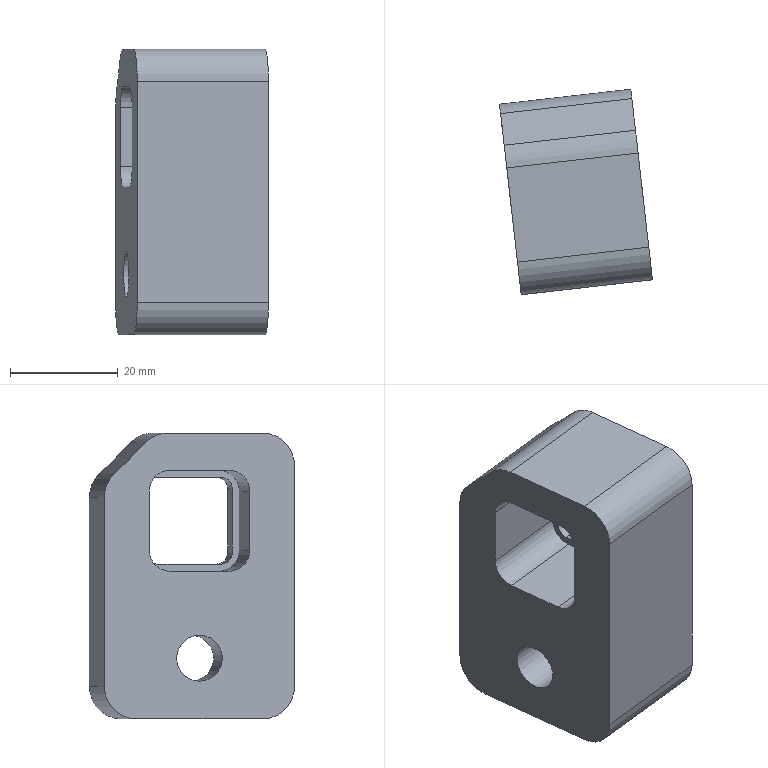Part | NX | features solid 2 | 1 solid | 32 faces | box 28.361 x 38.045 x 53 mm | volume 34321 mm3 | plane 17 | cylinder 15 | commonest cylinder face diameters 12 x5 4.08 x4 7.75 x4 8.5 x1 14 x1
STEP:
#1=CARTESIAN_POINT('',(3205.892,233.848,-55.317));
#2=VERTEX_POINT('',#1);
#3=CARTESIAN_POINT('',(3205.453,237.698,-51.442));
#4=VERTEX_POINT('',#3);
#5=CARTESIAN_POINT('',(3205.453,237.698,-55.317));
#6=DIRECTION('',(-0.9936,-0.1132,-0.000000001));
#7=DIRECTION('',(0.000000001,0.,-1.));
#8=AXIS2_PLACEMENT_3D('',#5,#6,#7);
#9=CIRCLE('',#8,3.875);
#10=EDGE_CURVE('',#2,#4,#9,.T.);
#11=ORIENTED_EDGE('',*,*,#10,.T.);
#12=CARTESIAN_POINT('',(3204.208,248.628,-51.442));
#13=VERTEX_POINT('',#12);
#14=CARTESIAN_POINT('',(3204.83,243.163,-51.442));
#15=DIRECTION('',(-0.1132,0.9936,0.));
#16=VECTOR('',#15,1000.);
#17=LINE('',#14,#16);
#18=EDGE_CURVE('',#4,#13,#17,.T.);
#19=ORIENTED_EDGE('',*,*,#18,.T.);
#20=CARTESIAN_POINT('',(3203.769,252.478,-55.317));
#21=VERTEX_POINT('',#20);
#22=CARTESIAN_POINT('',(3204.208,248.628,-55.317));
#23=DIRECTION('',(-0.9936,-0.1132,-0.000000001));
#24=DIRECTION('',(0.000000001,0.,-1.));
#25=AXIS2_PLACEMENT_3D('',#22,#23,#24);
#26=CIRCLE('',#25,3.875);
#27=EDGE_CURVE('',#13,#21,#26,.T.);
#28=ORIENTED_EDGE('',*,*,#27,.T.);
#29=CARTESIAN_POINT('',(3203.769,252.478,-66.317));
#30=VERTEX_POINT('',#29);
#31=CARTESIAN_POINT('',(3203.769,252.478,-61.567));
#32=DIRECTION('',(0.000000001,0.,-1.));
#33=VECTOR('',#32,1000.);
#34=LINE('',#31,#33);
#35=EDGE_CURVE('',#21,#30,#34,.T.);
#36=ORIENTED_EDGE('',*,*,#35,.T.);
#37=CARTESIAN_POINT('',(3204.208,248.628,-70.192));
#38=VERTEX_POINT('',#37);
#39=CARTESIAN_POINT('',(3204.208,248.628,-66.317));
#40=DIRECTION('',(0.9936,0.1132,0.000000001));
#41=DIRECTION('',(0.000000001,0.,-1.));
#42=AXIS2_PLACEMENT_3D('',#39,#40,#41);
#43=CIRCLE('',#42,3.875);
#44=EDGE_CURVE('',#38,#30,#43,.T.);
#45=ORIENTED_EDGE('',*,*,#44,.F.);
#46=CARTESIAN_POINT('',(3205.453,237.698,-70.192));
#47=VERTEX_POINT('',#46);
#48=CARTESIAN_POINT('',(3204.208,248.628,-70.192));
#49=DIRECTION('',(-0.1132,0.9936,0.));
#50=VECTOR('',#49,1000.);
#51=LINE('',#48,#50);
#52=EDGE_CURVE('',#47,#38,#51,.T.);
#53=ORIENTED_EDGE('',*,*,#52,.F.);
#54=CARTESIAN_POINT('',(3205.892,233.848,-66.317));
#55=VERTEX_POINT('',#54);
#56=CARTESIAN_POINT('',(3205.453,237.698,-66.317));
#57=DIRECTION('',(0.9936,0.1132,0.000000001));
#58=DIRECTION('',(0.000000001,0.,-1.));
#59=AXIS2_PLACEMENT_3D('',#56,#57,#58);
#60=CIRCLE('',#59,3.875);
#61=EDGE_CURVE('',#55,#47,#60,.T.);
#62=ORIENTED_EDGE('',*,*,#61,.F.);
#63=CARTESIAN_POINT('',(3205.892,233.848,-66.317));
#64=DIRECTION('',(0.000000001,0.,-1.));
#65=VECTOR('',#64,1000.);
#66=LINE('',#63,#65);
#67=EDGE_CURVE('',#2,#55,#66,.T.);
#68=ORIENTED_EDGE('',*,*,#67,.F.);
#69=EDGE_LOOP('',(#11,#19,#28,#36,#45,#53,#62,#68));
#70=FACE_BOUND('',#69,.T.);
#71=CARTESIAN_POINT('',(3205.74,235.175,-66.817));
#72=VERTEX_POINT('',#71);
#73=CARTESIAN_POINT('',(3205.74,235.175,-54.817));
#74=VERTEX_POINT('',#73);
#75=CARTESIAN_POINT('',(3205.74,235.175,-54.817));
#76=DIRECTION('',(-0.000000001,0.000000001,1.));
#77=VECTOR('',#76,1000.);
#78=LINE('',#75,#77);
#79=EDGE_CURVE('',#72,#74,#78,.T.);
#80=ORIENTED_EDGE('',*,*,#79,.F.);
#81=CARTESIAN_POINT('',(3205.51,237.202,-68.857));
#82=VERTEX_POINT('',#81);
#83=CARTESIAN_POINT('',(3205.51,237.202,-66.817));
#84=DIRECTION('',(-0.9936,-0.1132,-0.000000001));
#85=DIRECTION('',(0.000000001,0.,-1.));
#86=AXIS2_PLACEMENT_3D('',#83,#84,#85);
#87=CIRCLE('',#86,2.04);
#88=EDGE_CURVE('',#82,#72,#87,.T.);
#89=ORIENTED_EDGE('',*,*,#88,.F.);
#90=CARTESIAN_POINT('',(3204.151,249.124,-68.857));
#91=VERTEX_POINT('',#90);
#92=CARTESIAN_POINT('',(3205.51,237.202,-68.857));
#93=DIRECTION('',(0.1132,-0.9936,0.000000001));
#94=VECTOR('',#93,1000.);
#95=LINE('',#92,#94);
#96=EDGE_CURVE('',#91,#82,#95,.T.);
#97=ORIENTED_EDGE('',*,*,#96,.F.);
#98=CARTESIAN_POINT('',(3203.92,251.151,-66.817));
#99=VERTEX_POINT('',#98);
#100=CARTESIAN_POINT('',(3204.151,249.124,-66.817));
#101=DIRECTION('',(-0.9936,-0.1132,-0.000000001));
#102=DIRECTION('',(0.000000001,0.,-1.));
#103=AXIS2_PLACEMENT_3D('',#100,#101,#102);
#104=CIRCLE('',#103,2.04);
#105=EDGE_CURVE('',#99,#91,#104,.T.);
#106=ORIENTED_EDGE('',*,*,#105,.F.);
#107=CARTESIAN_POINT('',(3203.92,251.151,-54.817));
#108=VERTEX_POINT('',#107);
#109=CARTESIAN_POINT('',(3203.92,251.151,-66.317));
#110=DIRECTION('',(0.000000001,0.,-1.));
#111=VECTOR('',#110,1000.);
#112=LINE('',#109,#111);
#113=EDGE_CURVE('',#108,#99,#112,.T.);
#114=ORIENTED_EDGE('',*,*,#113,.F.);
#115=CARTESIAN_POINT('',(3204.151,249.124,-52.777));
#116=VERTEX_POINT('',#115);
#117=CARTESIAN_POINT('',(3204.151,249.124,-54.817));
#118=DIRECTION('',(-0.9936,-0.1132,-0.000000001));
#119=DIRECTION('',(0.000000001,0.,-1.));
#120=AXIS2_PLACEMENT_3D('',#117,#118,#119);
#121=CIRCLE('',#120,2.04);
#122=EDGE_CURVE('',#116,#108,#121,.T.);
#123=ORIENTED_EDGE('',*,*,#122,.F.);
#124=CARTESIAN_POINT('',(3205.51,237.202,-52.777));
#125=VERTEX_POINT('',#124);
#126=CARTESIAN_POINT('',(3204.151,249.124,-52.777));
#127=DIRECTION('',(-0.1132,0.9936,-0.000000001));
#128=VECTOR('',#127,1000.);
#129=LINE('',#126,#128);
#130=EDGE_CURVE('',#125,#116,#129,.T.);
#131=ORIENTED_EDGE('',*,*,#130,.F.);
#132=CARTESIAN_POINT('',(3205.51,237.202,-54.817));
#133=DIRECTION('',(-0.9936,-0.1132,-0.000000001));
#134=DIRECTION('',(0.000000001,0.,-1.));
#135=AXIS2_PLACEMENT_3D('',#132,#133,#134);
#136=CIRCLE('',#135,2.04);
#137=EDGE_CURVE('',#74,#125,#136,.T.);
#138=ORIENTED_EDGE('',*,*,#137,.F.);
#139=EDGE_LOOP('',(#80,#89,#97,#106,#114,#123,#131,#138));
#140=FACE_BOUND('',#139,.T.);
#141=CARTESIAN_POINT('',(3204.83,243.163,-61.567));
#142=DIRECTION('',(-0.9936,-0.1132,-0.000000001));
#143=DIRECTION('',(-0.1132,0.9936,0.));
#144=AXIS2_PLACEMENT_3D('',#141,#142,#143);
#145=PLANE('',#144);
#146=ADVANCED_FACE('',(#70,#140),#145,.T.);
#147=CARTESIAN_POINT('',(3187.94,241.239,-90.567));
#148=VERTEX_POINT('',#147);
#149=CARTESIAN_POINT('',(3187.94,241.239,-86.317));
#150=DIRECTION('',(-0.9936,-0.1132,-0.000000001));
#151=DIRECTION('',(0.000000001,0.,-1.));
#152=AXIS2_PLACEMENT_3D('',#149,#150,#151);
#153=CIRCLE('',#152,4.25);
#154=EDGE_CURVE('',#148,#148,#153,.T.);
#155=ORIENTED_EDGE('',*,*,#154,.F.);
#156=EDGE_LOOP('',(#155));
#157=FACE_BOUND('',#156,.T.);
#158=CARTESIAN_POINT('',(3189.27,229.564,-44.567));
#159=VERTEX_POINT('',#158);
#160=CARTESIAN_POINT('',(3187.279,247.036,-44.567));
#161=VERTEX_POINT('',#160);
#162=CARTESIAN_POINT('',(3189.921,223.851,-44.567));
#163=DIRECTION('',(-0.1132,0.9936,0.));
#164=VECTOR('',#163,1000.);
#165=LINE('',#162,#164);
#166=EDGE_CURVE('',#159,#161,#165,.T.);
#167=ORIENTED_EDGE('',*,*,#166,.T.);
#168=CARTESIAN_POINT('',(3186.799,251.252,-46.324));
#169=VERTEX_POINT('',#168);
#170=CARTESIAN_POINT('',(3187.279,247.036,-50.567));
#171=DIRECTION('',(0.9936,0.1132,0.000000001));
#172=DIRECTION('',(0.000000001,0.,-1.));
#173=AXIS2_PLACEMENT_3D('',#170,#171,#172);
#174=CIRCLE('',#173,6.);
#175=EDGE_CURVE('',#169,#161,#174,.T.);
#176=ORIENTED_EDGE('',*,*,#175,.F.);
#177=CARTESIAN_POINT('',(3186.129,257.128,-52.239));
#178=VERTEX_POINT('',#177);
#179=CARTESIAN_POINT('',(3186.506,253.817,-48.907));
#180=DIRECTION('',(0.08005,-0.7026,0.7071));
#181=VECTOR('',#180,1000.);
#182=LINE('',#179,#181);
#183=EDGE_CURVE('',#178,#169,#182,.T.);
#184=ORIENTED_EDGE('',*,*,#183,.F.);
#185=CARTESIAN_POINT('',(3185.93,258.874,-56.482));
#186=VERTEX_POINT('',#185);
#187=CARTESIAN_POINT('',(3186.609,252.913,-56.482));
#188=DIRECTION('',(0.9936,0.1132,0.000000001));
#189=DIRECTION('',(0.000000001,0.,-1.));
#190=AXIS2_PLACEMENT_3D('',#187,#188,#189);
#191=CIRCLE('',#190,6.);
#192=EDGE_CURVE('',#186,#178,#191,.T.);
#193=ORIENTED_EDGE('',*,*,#192,.F.);
#194=CARTESIAN_POINT('',(3185.93,258.874,-91.567));
#195=VERTEX_POINT('',#194);
#196=CARTESIAN_POINT('',(3185.93,258.874,-61.567));
#197=DIRECTION('',(-0.000000001,0.,1.));
#198=VECTOR('',#197,1000.);
#199=LINE('',#196,#198);
#200=EDGE_CURVE('',#195,#186,#199,.T.);
#201=ORIENTED_EDGE('',*,*,#200,.F.);
#202=CARTESIAN_POINT('',(3186.609,252.913,-97.567));
#203=VERTEX_POINT('',#202);
#204=CARTESIAN_POINT('',(3186.609,252.913,-91.567));
#205=DIRECTION('',(0.9936,0.1132,0.000000001));
#206=DIRECTION('',(0.000000001,0.,-1.));
#207=AXIS2_PLACEMENT_3D('',#204,#205,#206);
#208=CIRCLE('',#207,6.);
#209=EDGE_CURVE('',#203,#195,#208,.T.);
#210=ORIENTED_EDGE('',*,*,#209,.F.);
#211=CARTESIAN_POINT('',(3189.27,229.564,-97.567));
#212=VERTEX_POINT('',#211);
#213=CARTESIAN_POINT('',(3187.94,241.239,-97.567));
#214=DIRECTION('',(-0.1132,0.9936,0.));
#215=VECTOR('',#214,1000.);
#216=LINE('',#213,#215);
#217=EDGE_CURVE('',#212,#203,#216,.T.);
#218=ORIENTED_EDGE('',*,*,#217,.F.);
#219=CARTESIAN_POINT('',(3189.949,223.603,-91.567));
#220=VERTEX_POINT('',#219);
#221=CARTESIAN_POINT('',(3189.27,229.564,-91.567));
#222=DIRECTION('',(0.9936,0.1132,0.000000001));
#223=DIRECTION('',(0.000000001,0.,-1.));
#224=AXIS2_PLACEMENT_3D('',#221,#222,#223);
#225=CIRCLE('',#224,6.);
#226=EDGE_CURVE('',#220,#212,#225,.T.);
#227=ORIENTED_EDGE('',*,*,#226,.F.);
#228=CARTESIAN_POINT('',(3189.949,223.603,-50.567));
#229=VERTEX_POINT('',#228);
#230=CARTESIAN_POINT('',(3189.949,223.603,-61.567));
#231=DIRECTION('',(0.000000001,0.,-1.));
#232=VECTOR('',#231,1000.);
#233=LINE('',#230,#232);
#234=EDGE_CURVE('',#229,#220,#233,.T.);
#235=ORIENTED_EDGE('',*,*,#234,.F.);
#236=CARTESIAN_POINT('',(3189.27,229.564,-50.567));
#237=DIRECTION('',(0.9936,0.1132,0.000000001));
#238=DIRECTION('',(0.000000001,0.,-1.));
#239=AXIS2_PLACEMENT_3D('',#236,#237,#238);
#240=CIRCLE('',#239,6.);
#241=EDGE_CURVE('',#159,#229,#240,.T.);
#242=ORIENTED_EDGE('',*,*,#241,.F.);
#243=EDGE_LOOP('',(#167,#176,#184,#193,#201,#210,#218,#227,#235,#242));
#244=FACE_BOUND('',#243,.T.);
#245=CARTESIAN_POINT('',(3187.317,246.703,-70.192));
#246=VERTEX_POINT('',#245);
#247=CARTESIAN_POINT('',(3186.878,250.553,-66.317));
#248=VERTEX_POINT('',#247);
#249=CARTESIAN_POINT('',(3187.317,246.703,-66.317));
#250=DIRECTION('',(0.9936,0.1132,0.000000001));
#251=DIRECTION('',(0.000000001,0.,-1.));
#252=AXIS2_PLACEMENT_3D('',#249,#250,#251);
#253=CIRCLE('',#252,3.875);
#254=EDGE_CURVE('',#246,#248,#253,.T.);
#255=ORIENTED_EDGE('',*,*,#254,.T.);
#256=CARTESIAN_POINT('',(3186.878,250.553,-55.317));
#257=VERTEX_POINT('',#256);
#258=CARTESIAN_POINT('',(3186.878,250.553,-61.567));
#259=DIRECTION('',(0.000000001,0.,-1.));
#260=VECTOR('',#259,1000.);
#261=LINE('',#258,#260);
#262=EDGE_CURVE('',#257,#248,#261,.T.);
#263=ORIENTED_EDGE('',*,*,#262,.F.);
#264=CARTESIAN_POINT('',(3187.317,246.703,-51.442));
#265=VERTEX_POINT('',#264);
#266=CARTESIAN_POINT('',(3187.317,246.703,-55.317));
#267=DIRECTION('',(0.9936,0.1132,0.000000001));
#268=DIRECTION('',(0.000000001,0.,-1.));
#269=AXIS2_PLACEMENT_3D('',#266,#267,#268);
#270=CIRCLE('',#269,3.875);
#271=EDGE_CURVE('',#257,#265,#270,.T.);
#272=ORIENTED_EDGE('',*,*,#271,.T.);
#273=CARTESIAN_POINT('',(3188.562,235.774,-51.442));
#274=VERTEX_POINT('',#273);
#275=CARTESIAN_POINT('',(3187.94,241.239,-51.442));
#276=DIRECTION('',(-0.1132,0.9936,0.));
#277=VECTOR('',#276,1000.);
#278=LINE('',#275,#277);
#279=EDGE_CURVE('',#274,#265,#278,.T.);
#280=ORIENTED_EDGE('',*,*,#279,.F.);
#281=CARTESIAN_POINT('',(3189.001,231.924,-55.317));
#282=VERTEX_POINT('',#281);
#283=CARTESIAN_POINT('',(3188.562,235.774,-55.317));
#284=DIRECTION('',(0.9936,0.1132,0.000000001));
#285=DIRECTION('',(0.000000001,0.,-1.));
#286=AXIS2_PLACEMENT_3D('',#283,#284,#285);
#287=CIRCLE('',#286,3.875);
#288=EDGE_CURVE('',#274,#282,#287,.T.);
#289=ORIENTED_EDGE('',*,*,#288,.T.);
#290=CARTESIAN_POINT('',(3189.001,231.924,-66.317));
#291=VERTEX_POINT('',#290);
#292=CARTESIAN_POINT('',(3189.001,231.924,-61.567));
#293=DIRECTION('',(-0.000000001,0.,1.));
#294=VECTOR('',#293,1000.);
#295=LINE('',#292,#294);
#296=EDGE_CURVE('',#291,#282,#295,.T.);
#297=ORIENTED_EDGE('',*,*,#296,.F.);
#298=CARTESIAN_POINT('',(3188.562,235.774,-70.192));
#299=VERTEX_POINT('',#298);
#300=CARTESIAN_POINT('',(3188.562,235.774,-66.317));
#301=DIRECTION('',(0.9936,0.1132,0.000000001));
#302=DIRECTION('',(0.000000001,0.,-1.));
#303=AXIS2_PLACEMENT_3D('',#300,#301,#302);
#304=CIRCLE('',#303,3.875);
#305=EDGE_CURVE('',#291,#299,#304,.T.);
#306=ORIENTED_EDGE('',*,*,#305,.T.);
#307=CARTESIAN_POINT('',(3187.94,241.239,-70.192));
#308=DIRECTION('',(0.1132,-0.9936,0.));
#309=VECTOR('',#308,1000.);
#310=LINE('',#307,#309);
#311=EDGE_CURVE('',#246,#299,#310,.T.);
#312=ORIENTED_EDGE('',*,*,#311,.F.);
#313=EDGE_LOOP('',(#255,#263,#272,#280,#289,#297,#306,#312));
#314=FACE_BOUND('',#313,.T.);
#315=CARTESIAN_POINT('',(3187.94,241.239,-61.567));
#316=DIRECTION('',(-0.9936,-0.1132,-0.000000001));
#317=DIRECTION('',(-0.1132,0.9936,0.));
#318=AXIS2_PLACEMENT_3D('',#315,#316,#317);
#319=PLANE('',#318);
#320=ADVANCED_FACE('',(#157,#244,#314),#319,.T.);
#321=CARTESIAN_POINT('',(3212.961,238.051,-52.777));
#322=VERTEX_POINT('',#321);
#323=CARTESIAN_POINT('',(3211.603,249.973,-52.777));
#324=VERTEX_POINT('',#323);
#325=CARTESIAN_POINT('',(3214.263,226.624,-52.777));
#326=DIRECTION('',(-0.1132,0.9936,-0.000000001));
#327=VECTOR('',#326,1000.);
#328=LINE('',#325,#327);
#329=EDGE_CURVE('',#322,#324,#328,.T.);
#330=ORIENTED_EDGE('',*,*,#329,.T.);
#331=CARTESIAN_POINT('',(3211.372,252.,-54.817));
#332=VERTEX_POINT('',#331);
#333=CARTESIAN_POINT('',(3211.603,249.973,-54.817));
#334=DIRECTION('',(-0.9936,-0.1132,-0.000000001));
#335=DIRECTION('',(-0.000000001,0.,1.));
#336=AXIS2_PLACEMENT_3D('',#333,#334,#335);
#337=CIRCLE('',#336,2.04);
#338=EDGE_CURVE('',#324,#332,#337,.T.);
#339=ORIENTED_EDGE('',*,*,#338,.T.);
#340=CARTESIAN_POINT('',(3211.372,252.,-66.817));
#341=VERTEX_POINT('',#340);
#342=CARTESIAN_POINT('',(3211.372,252.,-70.067));
#343=DIRECTION('',(0.000000001,0.,-1.));
#344=VECTOR('',#343,1000.);
#345=LINE('',#342,#344);
#346=EDGE_CURVE('',#332,#341,#345,.T.);
#347=ORIENTED_EDGE('',*,*,#346,.T.);
#348=CARTESIAN_POINT('',(3211.603,249.973,-68.857));
#349=VERTEX_POINT('',#348);
#350=CARTESIAN_POINT('',(3211.603,249.973,-66.817));
#351=DIRECTION('',(-0.9936,-0.1132,-0.000000001));
#352=DIRECTION('',(-0.000000001,0.,1.));
#353=AXIS2_PLACEMENT_3D('',#350,#351,#352);
#354=CIRCLE('',#353,2.04);
#355=EDGE_CURVE('',#341,#349,#354,.T.);
#356=ORIENTED_EDGE('',*,*,#355,.T.);
#357=CARTESIAN_POINT('',(3212.961,238.051,-68.857));
#358=VERTEX_POINT('',#357);
#359=CARTESIAN_POINT('',(3214.263,226.624,-68.857));
#360=DIRECTION('',(0.1132,-0.9936,0.000000001));
#361=VECTOR('',#360,1000.);
#362=LINE('',#359,#361);
#363=EDGE_CURVE('',#349,#358,#362,.T.);
#364=ORIENTED_EDGE('',*,*,#363,.T.);
#365=CARTESIAN_POINT('',(3213.192,236.024,-66.817));
#366=VERTEX_POINT('',#365);
#367=CARTESIAN_POINT('',(3212.961,238.051,-66.817));
#368=DIRECTION('',(-0.9936,-0.1132,-0.000000001));
#369=DIRECTION('',(-0.000000001,0.,1.));
#370=AXIS2_PLACEMENT_3D('',#367,#368,#369);
#371=CIRCLE('',#370,2.04);
#372=EDGE_CURVE('',#358,#366,#371,.T.);
#373=ORIENTED_EDGE('',*,*,#372,.T.);
#374=CARTESIAN_POINT('',(3213.192,236.024,-54.817));
#375=VERTEX_POINT('',#374);
#376=CARTESIAN_POINT('',(3213.192,236.024,-70.067));
#377=DIRECTION('',(-0.000000001,0.000000001,1.));
#378=VECTOR('',#377,1000.);
#379=LINE('',#376,#378);
#380=EDGE_CURVE('',#366,#375,#379,.T.);
#381=ORIENTED_EDGE('',*,*,#380,.T.);
#382=CARTESIAN_POINT('',(3212.961,238.051,-54.817));
#383=DIRECTION('',(-0.9936,-0.1132,-0.000000001));
#384=DIRECTION('',(-0.000000001,0.,1.));
#385=AXIS2_PLACEMENT_3D('',#382,#383,#384);
#386=CIRCLE('',#385,2.04);
#387=EDGE_CURVE('',#375,#322,#386,.T.);
#388=ORIENTED_EDGE('',*,*,#387,.T.);
#389=EDGE_LOOP('',(#330,#339,#347,#356,#364,#373,#381,#388));
#390=FACE_BOUND('',#389,.T.);
#391=CARTESIAN_POINT('',(3214.291,226.376,-91.567));
#392=VERTEX_POINT('',#391);
#393=CARTESIAN_POINT('',(3214.291,226.376,-50.567));
#394=VERTEX_POINT('',#393);
#395=CARTESIAN_POINT('',(3214.291,226.376,-70.067));
#396=DIRECTION('',(-0.000000001,0.,1.));
#397=VECTOR('',#396,1000.);
#398=LINE('',#395,#397);
#399=EDGE_CURVE('',#392,#394,#398,.T.);
#400=ORIENTED_EDGE('',*,*,#399,.F.);
#401=CARTESIAN_POINT('',(3213.612,232.338,-97.567));
#402=VERTEX_POINT('',#401);
#403=CARTESIAN_POINT('',(3213.612,232.338,-91.567));
#404=DIRECTION('',(-0.9936,-0.1132,-0.000000001));
#405=DIRECTION('',(-0.000000001,0.,1.));
#406=AXIS2_PLACEMENT_3D('',#403,#404,#405);
#407=CIRCLE('',#406,6.);
#408=EDGE_CURVE('',#402,#392,#407,.T.);
#409=ORIENTED_EDGE('',*,*,#408,.F.);
#410=CARTESIAN_POINT('',(3210.952,255.686,-97.567));
#411=VERTEX_POINT('',#410);
#412=CARTESIAN_POINT('',(3214.263,226.624,-97.567));
#413=DIRECTION('',(-0.1132,0.9936,0.));
#414=VECTOR('',#413,1000.);
#415=LINE('',#412,#414);
#416=EDGE_CURVE('',#402,#411,#415,.T.);
#417=ORIENTED_EDGE('',*,*,#416,.T.);
#418=CARTESIAN_POINT('',(3210.273,261.648,-91.567));
#419=VERTEX_POINT('',#418);
#420=CARTESIAN_POINT('',(3210.952,255.686,-91.567));
#421=DIRECTION('',(-0.9936,-0.1132,-0.000000001));
#422=DIRECTION('',(-0.000000001,0.,1.));
#423=AXIS2_PLACEMENT_3D('',#420,#421,#422);
#424=CIRCLE('',#423,6.);
#425=EDGE_CURVE('',#419,#411,#424,.T.);
#426=ORIENTED_EDGE('',*,*,#425,.F.);
#427=CARTESIAN_POINT('',(3210.273,261.648,-56.482));
#428=VERTEX_POINT('',#427);
#429=CARTESIAN_POINT('',(3210.273,261.648,-70.067));
#430=DIRECTION('',(0.000000001,0.,-1.));
#431=VECTOR('',#430,1000.);
#432=LINE('',#429,#431);
#433=EDGE_CURVE('',#428,#419,#432,.T.);
#434=ORIENTED_EDGE('',*,*,#433,.F.);
#435=CARTESIAN_POINT('',(3210.472,259.902,-52.239));
#436=VERTEX_POINT('',#435);
#437=CARTESIAN_POINT('',(3210.952,255.686,-56.482));
#438=DIRECTION('',(-0.9936,-0.1132,-0.000000001));
#439=DIRECTION('',(-0.000000001,0.,1.));
#440=AXIS2_PLACEMENT_3D('',#437,#438,#439);
#441=CIRCLE('',#440,6.);
#442=EDGE_CURVE('',#436,#428,#441,.T.);
#443=ORIENTED_EDGE('',*,*,#442,.F.);
#444=CARTESIAN_POINT('',(3211.141,254.025,-46.324));
#445=VERTEX_POINT('',#444);
#446=CARTESIAN_POINT('',(3211.358,252.12,-44.407));
#447=DIRECTION('',(-0.08005,0.7026,-0.7071));
#448=VECTOR('',#447,1000.);
#449=LINE('',#446,#448);
#450=EDGE_CURVE('',#445,#436,#449,.T.);
#451=ORIENTED_EDGE('',*,*,#450,.F.);
#452=CARTESIAN_POINT('',(3211.622,249.81,-44.567));
#453=VERTEX_POINT('',#452);
#454=CARTESIAN_POINT('',(3211.622,249.81,-50.567));
#455=DIRECTION('',(-0.9936,-0.1132,-0.000000001));
#456=DIRECTION('',(-0.000000001,0.,1.));
#457=AXIS2_PLACEMENT_3D('',#454,#455,#456);
#458=CIRCLE('',#457,6.);
#459=EDGE_CURVE('',#453,#445,#458,.T.);
#460=ORIENTED_EDGE('',*,*,#459,.F.);
#461=CARTESIAN_POINT('',(3213.612,232.338,-44.567));
#462=VERTEX_POINT('',#461);
#463=CARTESIAN_POINT('',(3214.263,226.624,-44.567));
#464=DIRECTION('',(-0.1132,0.9936,0.));
#465=VECTOR('',#464,1000.);
#466=LINE('',#463,#465);
#467=EDGE_CURVE('',#462,#453,#466,.T.);
#468=ORIENTED_EDGE('',*,*,#467,.F.);
#469=CARTESIAN_POINT('',(3213.612,232.338,-50.567));
#470=DIRECTION('',(-0.9936,-0.1132,-0.000000001));
#471=DIRECTION('',(-0.000000001,0.,1.));
#472=AXIS2_PLACEMENT_3D('',#469,#470,#471);
#473=CIRCLE('',#472,6.);
#474=EDGE_CURVE('',#394,#462,#473,.T.);
#475=ORIENTED_EDGE('',*,*,#474,.F.);
#476=EDGE_LOOP('',(#400,#409,#417,#426,#434,#443,#451,#460,#468,#475));
#477=FACE_BOUND('',#476,.T.);
#478=CARTESIAN_POINT('',(3212.282,244.012,-79.317));
#479=VERTEX_POINT('',#478);
#480=CARTESIAN_POINT('',(3212.282,244.012,-86.317));
#481=DIRECTION('',(-0.9936,-0.1132,-0.000000001));
#482=DIRECTION('',(-0.000000001,0.,1.));
#483=AXIS2_PLACEMENT_3D('',#480,#481,#482);
#484=CIRCLE('',#483,7.);
#485=EDGE_CURVE('',#479,#479,#484,.T.);
#486=ORIENTED_EDGE('',*,*,#485,.T.);
#487=EDGE_LOOP('',(#486));
#488=FACE_BOUND('',#487,.T.);
#489=CARTESIAN_POINT('',(3214.263,226.624,-70.067));
#490=DIRECTION('',(0.9936,0.1132,0.000000001));
#491=DIRECTION('',(0.1132,-0.9936,0.));
#492=AXIS2_PLACEMENT_3D('',#489,#490,#491);
#493=PLANE('',#492);
#494=ADVANCED_FACE('',(#390,#477,#488),#493,.T.);
#495=ORIENTED_EDGE('',*,*,#200,.T.);
#496=CARTESIAN_POINT('',(3203.318,260.855,-56.482));
#497=DIRECTION('',(-0.9936,-0.1132,-0.000000001));
#498=VECTOR('',#497,1000.);
#499=LINE('',#496,#498);
#500=EDGE_CURVE('',#428,#186,#499,.T.);
#501=ORIENTED_EDGE('',*,*,#500,.F.);
#502=ORIENTED_EDGE('',*,*,#433,.T.);
#503=CARTESIAN_POINT('',(3203.318,260.855,-91.567));
#504=DIRECTION('',(0.9936,0.1132,0.000000001));
#505=VECTOR('',#504,1000.);
#506=LINE('',#503,#505);
#507=EDGE_CURVE('',#195,#419,#506,.T.);
#508=ORIENTED_EDGE('',*,*,#507,.F.);
#509=EDGE_LOOP('',(#495,#501,#502,#508));
#510=FACE_BOUND('',#509,.T.);
#511=CARTESIAN_POINT('',(3203.318,260.855,-70.067));
#512=DIRECTION('',(-0.1132,0.9936,0.));
#513=DIRECTION('',(0.9936,0.1132,0.000000001));
#514=AXIS2_PLACEMENT_3D('',#511,#512,#513);
#515=PLANE('',#514);
#516=ADVANCED_FACE('',(#510),#515,.T.);
#517=ORIENTED_EDGE('',*,*,#217,.T.);
#518=CARTESIAN_POINT('',(3203.997,254.894,-97.567));
#519=DIRECTION('',(-0.9936,-0.1132,-0.000000001));
#520=VECTOR('',#519,1000.);
#521=LINE('',#518,#520);
#522=EDGE_CURVE('',#411,#203,#521,.T.);
#523=ORIENTED_EDGE('',*,*,#522,.F.);
#524=ORIENTED_EDGE('',*,*,#416,.F.);
#525=CARTESIAN_POINT('',(3206.657,231.545,-97.567));
#526=DIRECTION('',(0.9936,0.1132,0.000000001));
#527=VECTOR('',#526,1000.);
#528=LINE('',#525,#527);
#529=EDGE_CURVE('',#212,#402,#528,.T.);
#530=ORIENTED_EDGE('',*,*,#529,.F.);
#531=EDGE_LOOP('',(#517,#523,#524,#530));
#532=FACE_BOUND('',#531,.T.);
#533=CARTESIAN_POINT('',(3207.308,225.832,-97.567));
#534=DIRECTION('',(0.000000001,0.,-1.));
#535=DIRECTION('',(0.1132,-0.9936,0.));
#536=AXIS2_PLACEMENT_3D('',#533,#534,#535);
#537=PLANE('',#536);
#538=ADVANCED_FACE('',(#532),#537,.T.);
#539=ORIENTED_EDGE('',*,*,#467,.T.);
#540=CARTESIAN_POINT('',(3204.667,249.017,-44.567));
#541=DIRECTION('',(0.9936,0.1132,0.000000001));
#542=VECTOR('',#541,1000.);
#543=LINE('',#540,#542);
#544=EDGE_CURVE('',#161,#453,#543,.T.);
#545=ORIENTED_EDGE('',*,*,#544,.F.);
#546=ORIENTED_EDGE('',*,*,#166,.F.);
#547=CARTESIAN_POINT('',(3206.657,231.545,-44.567));
#548=DIRECTION('',(-0.9936,-0.1132,-0.000000001));
#549=VECTOR('',#548,1000.);
#550=LINE('',#547,#549);
#551=EDGE_CURVE('',#462,#159,#550,.T.);
#552=ORIENTED_EDGE('',*,*,#551,.F.);
#553=EDGE_LOOP('',(#539,#545,#546,#552));
#554=FACE_BOUND('',#553,.T.);
#555=CARTESIAN_POINT('',(3207.308,225.832,-44.567));
#556=DIRECTION('',(-0.000000001,0.,1.));
#557=DIRECTION('',(-0.1132,0.9936,0.));
#558=AXIS2_PLACEMENT_3D('',#555,#556,#557);
#559=PLANE('',#558);
#560=ADVANCED_FACE('',(#554),#559,.T.);
#561=ORIENTED_EDGE('',*,*,#234,.T.);
#562=CARTESIAN_POINT('',(3207.336,225.584,-91.567));
#563=DIRECTION('',(-0.9936,-0.1132,-0.000000001));
#564=VECTOR('',#563,1000.);
#565=LINE('',#562,#564);
#566=EDGE_CURVE('',#392,#220,#565,.T.);
#567=ORIENTED_EDGE('',*,*,#566,.F.);
#568=ORIENTED_EDGE('',*,*,#399,.T.);
#569=CARTESIAN_POINT('',(3207.336,225.584,-50.567));
#570=DIRECTION('',(0.9936,0.1132,0.000000001));
#571=VECTOR('',#570,1000.);
#572=LINE('',#569,#571);
#573=EDGE_CURVE('',#229,#394,#572,.T.);
#574=ORIENTED_EDGE('',*,*,#573,.F.);
#575=EDGE_LOOP('',(#561,#567,#568,#574));
#576=FACE_BOUND('',#575,.T.);
#577=CARTESIAN_POINT('',(3207.336,225.584,-70.067));
#578=DIRECTION('',(0.1132,-0.9936,0.));
#579=DIRECTION('',(-0.9936,-0.1132,-0.000000001));
#580=AXIS2_PLACEMENT_3D('',#577,#578,#579);
#581=PLANE('',#580);
#582=ADVANCED_FACE('',(#576),#581,.T.);
#583=ORIENTED_EDGE('',*,*,#183,.T.);
#584=CARTESIAN_POINT('',(3204.186,253.233,-46.324));
#585=DIRECTION('',(-0.9936,-0.1132,-0.000000001));
#586=VECTOR('',#585,1000.);
#587=LINE('',#584,#586);
#588=EDGE_CURVE('',#445,#169,#587,.T.);
#589=ORIENTED_EDGE('',*,*,#588,.F.);
#590=ORIENTED_EDGE('',*,*,#450,.T.);
#591=CARTESIAN_POINT('',(3203.517,259.109,-52.239));
#592=DIRECTION('',(0.9936,0.1132,0.000000001));
#593=VECTOR('',#592,1000.);
#594=LINE('',#591,#593);
#595=EDGE_CURVE('',#178,#436,#594,.T.);
#596=ORIENTED_EDGE('',*,*,#595,.F.);
#597=EDGE_LOOP('',(#583,#589,#590,#596));
#598=FACE_BOUND('',#597,.T.);
#599=CARTESIAN_POINT('',(3204.361,251.7,-44.782));
#600=DIRECTION('',(0.08005,-0.7026,-0.7071));
#601=DIRECTION('',(0.9936,0.1132,0.000000001));
#602=AXIS2_PLACEMENT_3D('',#599,#600,#601);
#603=PLANE('',#602);
#604=ADVANCED_FACE('',(#598),#603,.F.);
#605=CARTESIAN_POINT('',(3201.368,247.046,-86.317));
#606=VERTEX_POINT('',#605);
#607=CARTESIAN_POINT('',(3201.85,242.823,-86.317));
#608=DIRECTION('',(0.9936,0.1132,0.000000001));
#609=DIRECTION('',(-0.1132,0.9936,0.));
#610=AXIS2_PLACEMENT_3D('',#607,#608,#609);
#611=CIRCLE('',#610,4.25);
#612=EDGE_CURVE('',#606,#606,#611,.T.);
#613=ORIENTED_EDGE('',*,*,#612,.T.);
#614=EDGE_LOOP('',(#613));
#615=FACE_BOUND('',#614,.T.);
#616=ORIENTED_EDGE('',*,*,#154,.T.);
#617=EDGE_LOOP('',(#616));
#618=FACE_BOUND('',#617,.T.);
#619=CARTESIAN_POINT('',(3247.554,248.031,-86.317));
#620=DIRECTION('',(-0.9936,-0.1132,-0.000000001));
#621=DIRECTION('',(0.000000001,0.,-1.));
#622=AXIS2_PLACEMENT_3D('',#619,#620,#621);
#623=CYLINDRICAL_SURFACE('',#622,4.25);
#624=ADVANCED_FACE('',(#615,#618),#623,.F.);
#625=ORIENTED_EDGE('',*,*,#485,.F.);
#626=EDGE_LOOP('',(#625));
#627=FACE_BOUND('',#626,.T.);
#628=CARTESIAN_POINT('',(3201.85,242.823,-79.317));
#629=VERTEX_POINT('',#628);
#630=CARTESIAN_POINT('',(3201.85,242.823,-86.317));
#631=DIRECTION('',(-0.9936,-0.1132,-0.000000001));
#632=DIRECTION('',(-0.000000001,0.,1.));
#633=AXIS2_PLACEMENT_3D('',#630,#631,#632);
#634=CIRCLE('',#633,7.);
#635=EDGE_CURVE('',#629,#629,#634,.T.);
#636=ORIENTED_EDGE('',*,*,#635,.T.);
#637=EDGE_LOOP('',(#636));
#638=FACE_BOUND('',#637,.T.);
#639=CARTESIAN_POINT('',(3223.708,245.314,-86.317));
#640=DIRECTION('',(-0.9936,-0.1132,-0.000000001));
#641=DIRECTION('',(-0.1132,0.9936,0.));
#642=AXIS2_PLACEMENT_3D('',#639,#640,#641);
#643=CYLINDRICAL_SURFACE('',#642,7.);
#644=ADVANCED_FACE('',(#627,#638),#643,.F.);
#645=ORIENTED_EDGE('',*,*,#612,.F.);
#646=EDGE_LOOP('',(#645));
#647=FACE_BOUND('',#646,.T.);
#648=ORIENTED_EDGE('',*,*,#635,.F.);
#649=EDGE_LOOP('',(#648));
#650=FACE_BOUND('',#649,.T.);
#651=CARTESIAN_POINT('',(3201.85,242.823,-86.317));
#652=DIRECTION('',(-0.9936,-0.1132,-0.000000001));
#653=DIRECTION('',(-0.1132,0.9936,0.));
#654=AXIS2_PLACEMENT_3D('',#651,#652,#653);
#655=PLANE('',#654);
#656=ADVANCED_FACE('',(#647,#650),#655,.F.);
#657=ORIENTED_EDGE('',*,*,#271,.F.);
#658=CARTESIAN_POINT('',(3296.171,263.006,-55.317));
#659=DIRECTION('',(0.9936,0.1132,0.000000001));
#660=VECTOR('',#659,1000.);
#661=LINE('',#658,#660);
#662=EDGE_CURVE('',#257,#21,#661,.T.);
#663=ORIENTED_EDGE('',*,*,#662,.T.);
#664=ORIENTED_EDGE('',*,*,#27,.F.);
#665=CARTESIAN_POINT('',(3296.61,259.156,-51.442));
#666=DIRECTION('',(0.9936,0.1132,0.000000001));
#667=VECTOR('',#666,1000.);
#668=LINE('',#665,#667);
#669=EDGE_CURVE('',#265,#13,#668,.T.);
#670=ORIENTED_EDGE('',*,*,#669,.F.);
#671=EDGE_LOOP('',(#657,#663,#664,#670));
#672=FACE_BOUND('',#671,.T.);
#673=CARTESIAN_POINT('',(3296.61,259.156,-55.317));
#674=DIRECTION('',(-0.9936,-0.1132,-0.000000001));
#675=DIRECTION('',(0.1132,-0.9936,0.));
#676=AXIS2_PLACEMENT_3D('',#673,#674,#675);
#677=CYLINDRICAL_SURFACE('',#676,3.875);
#678=ADVANCED_FACE('',(#672),#677,.F.);
#679=ORIENTED_EDGE('',*,*,#254,.F.);
#680=CARTESIAN_POINT('',(3296.61,259.156,-70.192));
#681=DIRECTION('',(0.9936,0.1132,0.000000001));
#682=VECTOR('',#681,1000.);
#683=LINE('',#680,#682);
#684=EDGE_CURVE('',#246,#38,#683,.T.);
#685=ORIENTED_EDGE('',*,*,#684,.T.);
#686=ORIENTED_EDGE('',*,*,#44,.T.);
#687=CARTESIAN_POINT('',(3296.171,263.006,-66.317));
#688=DIRECTION('',(0.9936,0.1132,0.000000001));
#689=VECTOR('',#688,1000.);
#690=LINE('',#687,#689);
#691=EDGE_CURVE('',#248,#30,#690,.T.);
#692=ORIENTED_EDGE('',*,*,#691,.F.);
#693=EDGE_LOOP('',(#679,#685,#686,#692));
#694=FACE_BOUND('',#693,.T.);
#695=CARTESIAN_POINT('',(3296.61,259.156,-66.317));
#696=DIRECTION('',(-0.9936,-0.1132,-0.000000001));
#697=DIRECTION('',(0.1132,-0.9936,0.));
#698=AXIS2_PLACEMENT_3D('',#695,#696,#697);
#699=CYLINDRICAL_SURFACE('',#698,3.875);
#700=ADVANCED_FACE('',(#694),#699,.F.);
#701=CARTESIAN_POINT('',(3298.294,244.376,-66.317));
#702=DIRECTION('',(0.9936,0.1132,0.000000001));
#703=VECTOR('',#702,1000.);
#704=LINE('',#701,#703);
#705=EDGE_CURVE('',#291,#55,#704,.T.);
#706=ORIENTED_EDGE('',*,*,#705,.F.);
#707=ORIENTED_EDGE('',*,*,#296,.T.);
#708=CARTESIAN_POINT('',(3298.294,244.376,-55.317));
#709=DIRECTION('',(0.9936,0.1132,0.000000001));
#710=VECTOR('',#709,1000.);
#711=LINE('',#708,#710);
#712=EDGE_CURVE('',#282,#2,#711,.T.);
#713=ORIENTED_EDGE('',*,*,#712,.T.);
#714=ORIENTED_EDGE('',*,*,#67,.T.);
#715=EDGE_LOOP('',(#706,#707,#713,#714));
#716=FACE_BOUND('',#715,.T.);
#717=CARTESIAN_POINT('',(3298.294,244.376,-66.317));
#718=DIRECTION('',(-0.1132,0.9936,0.));
#719=DIRECTION('',(-0.9936,-0.1132,-0.000000001));
#720=AXIS2_PLACEMENT_3D('',#717,#718,#719);
#721=PLANE('',#720);
#722=ADVANCED_FACE('',(#716),#721,.T.);
#723=CARTESIAN_POINT('',(3297.855,248.226,-51.442));
#724=DIRECTION('',(0.9936,0.1132,0.000000001));
#725=VECTOR('',#724,1000.);
#726=LINE('',#723,#725);
#727=EDGE_CURVE('',#274,#4,#726,.T.);
#728=ORIENTED_EDGE('',*,*,#727,.F.);
#729=ORIENTED_EDGE('',*,*,#279,.T.);
#730=ORIENTED_EDGE('',*,*,#669,.T.);
#731=ORIENTED_EDGE('',*,*,#18,.F.);
#732=EDGE_LOOP('',(#728,#729,#730,#731));
#733=FACE_BOUND('',#732,.T.);
#734=CARTESIAN_POINT('',(3297.855,248.226,-51.442));
#735=DIRECTION('',(0.000000001,0.,-1.));
#736=DIRECTION('',(-0.284,0.9588,0.));
#737=AXIS2_PLACEMENT_3D('',#734,#735,#736);
#738=PLANE('',#737);
#739=ADVANCED_FACE('',(#733),#738,.T.);
#740=ORIENTED_EDGE('',*,*,#305,.F.);
#741=ORIENTED_EDGE('',*,*,#705,.T.);
#742=ORIENTED_EDGE('',*,*,#61,.T.);
#743=CARTESIAN_POINT('',(3297.855,248.226,-70.192));
#744=DIRECTION('',(0.9936,0.1132,0.000000001));
#745=VECTOR('',#744,1000.);
#746=LINE('',#743,#745);
#747=EDGE_CURVE('',#299,#47,#746,.T.);
#748=ORIENTED_EDGE('',*,*,#747,.F.);
#749=EDGE_LOOP('',(#740,#741,#742,#748));
#750=FACE_BOUND('',#749,.T.);
#751=CARTESIAN_POINT('',(3297.855,248.226,-66.317));
#752=DIRECTION('',(-0.9936,-0.1132,-0.000000001));
#753=DIRECTION('',(0.1132,-0.9936,0.));
#754=AXIS2_PLACEMENT_3D('',#751,#752,#753);
#755=CYLINDRICAL_SURFACE('',#754,3.875);
#756=ADVANCED_FACE('',(#750),#755,.F.);
#757=ORIENTED_EDGE('',*,*,#662,.F.);
#758=ORIENTED_EDGE('',*,*,#262,.T.);
#759=ORIENTED_EDGE('',*,*,#691,.T.);
#760=ORIENTED_EDGE('',*,*,#35,.F.);
#761=EDGE_LOOP('',(#757,#758,#759,#760));
#762=FACE_BOUND('',#761,.T.);
#763=CARTESIAN_POINT('',(3296.171,263.006,-55.317));
#764=DIRECTION('',(0.1132,-0.9936,0.));
#765=DIRECTION('',(0.9936,0.1132,0.000000001));
#766=AXIS2_PLACEMENT_3D('',#763,#764,#765);
#767=PLANE('',#766);
#768=ADVANCED_FACE('',(#762),#767,.T.);
#769=ORIENTED_EDGE('',*,*,#684,.F.);
#770=ORIENTED_EDGE('',*,*,#311,.T.);
#771=ORIENTED_EDGE('',*,*,#747,.T.);
#772=ORIENTED_EDGE('',*,*,#52,.T.);
#773=EDGE_LOOP('',(#769,#770,#771,#772));
#774=FACE_BOUND('',#773,.T.);
#775=CARTESIAN_POINT('',(3296.61,259.156,-70.192));
#776=DIRECTION('',(-0.000000001,0.,1.));
#777=DIRECTION('',(0.284,-0.9588,0.));
#778=AXIS2_PLACEMENT_3D('',#775,#776,#777);
#779=PLANE('',#778);
#780=ADVANCED_FACE('',(#774),#779,.T.);
#781=ORIENTED_EDGE('',*,*,#288,.F.);
#782=ORIENTED_EDGE('',*,*,#727,.T.);
#783=ORIENTED_EDGE('',*,*,#10,.F.);
#784=ORIENTED_EDGE('',*,*,#712,.F.);
#785=EDGE_LOOP('',(#781,#782,#783,#784));
#786=FACE_BOUND('',#785,.T.);
#787=CARTESIAN_POINT('',(3297.855,248.226,-55.317));
#788=DIRECTION('',(-0.9936,-0.1132,-0.000000001));
#789=DIRECTION('',(0.1132,-0.9936,0.));
#790=AXIS2_PLACEMENT_3D('',#787,#788,#789);
#791=CYLINDRICAL_SURFACE('',#790,3.875);
#792=ADVANCED_FACE('',(#786),#791,.F.);
#793=ORIENTED_EDGE('',*,*,#474,.T.);
#794=ORIENTED_EDGE('',*,*,#551,.T.);
#795=ORIENTED_EDGE('',*,*,#241,.T.);
#796=ORIENTED_EDGE('',*,*,#573,.T.);
#797=EDGE_LOOP('',(#793,#794,#795,#796));
#798=FACE_BOUND('',#797,.T.);
#799=CARTESIAN_POINT('',(3206.657,231.545,-50.567));
#800=DIRECTION('',(-0.9936,-0.1132,-0.000000001));
#801=DIRECTION('',(-0.1132,0.9936,0.));
#802=AXIS2_PLACEMENT_3D('',#799,#800,#801);
#803=CYLINDRICAL_SURFACE('',#802,6.);
#804=ADVANCED_FACE('',(#798),#803,.T.);
#805=ORIENTED_EDGE('',*,*,#226,.T.);
#806=ORIENTED_EDGE('',*,*,#529,.T.);
#807=ORIENTED_EDGE('',*,*,#408,.T.);
#808=ORIENTED_EDGE('',*,*,#566,.T.);
#809=EDGE_LOOP('',(#805,#806,#807,#808));
#810=FACE_BOUND('',#809,.T.);
#811=CARTESIAN_POINT('',(3206.657,231.545,-91.567));
#812=DIRECTION('',(0.9936,0.1132,0.000000001));
#813=DIRECTION('',(0.1132,-0.9936,0.));
#814=AXIS2_PLACEMENT_3D('',#811,#812,#813);
#815=CYLINDRICAL_SURFACE('',#814,6.);
#816=ADVANCED_FACE('',(#810),#815,.T.);
#817=ORIENTED_EDGE('',*,*,#425,.T.);
#818=ORIENTED_EDGE('',*,*,#522,.T.);
#819=ORIENTED_EDGE('',*,*,#209,.T.);
#820=ORIENTED_EDGE('',*,*,#507,.T.);
#821=EDGE_LOOP('',(#817,#818,#819,#820));
#822=FACE_BOUND('',#821,.T.);
#823=CARTESIAN_POINT('',(3203.997,254.894,-91.567));
#824=DIRECTION('',(-0.9936,-0.1132,-0.000000001));
#825=DIRECTION('',(-0.1132,0.9936,0.));
#826=AXIS2_PLACEMENT_3D('',#823,#824,#825);
#827=CYLINDRICAL_SURFACE('',#826,6.);
#828=ADVANCED_FACE('',(#822),#827,.T.);
#829=ORIENTED_EDGE('',*,*,#442,.T.);
#830=ORIENTED_EDGE('',*,*,#500,.T.);
#831=ORIENTED_EDGE('',*,*,#192,.T.);
#832=ORIENTED_EDGE('',*,*,#595,.T.);
#833=EDGE_LOOP('',(#829,#830,#831,#832));
#834=FACE_BOUND('',#833,.T.);
#835=CARTESIAN_POINT('',(3203.997,254.894,-56.482));
#836=DIRECTION('',(0.9936,0.1132,0.000000001));
#837=DIRECTION('',(0.1132,-0.9936,0.));
#838=AXIS2_PLACEMENT_3D('',#835,#836,#837);
#839=CYLINDRICAL_SURFACE('',#838,6.);
#840=ADVANCED_FACE('',(#834),#839,.T.);
#841=ORIENTED_EDGE('',*,*,#175,.T.);
#842=ORIENTED_EDGE('',*,*,#544,.T.);
#843=ORIENTED_EDGE('',*,*,#459,.T.);
#844=ORIENTED_EDGE('',*,*,#588,.T.);
#845=EDGE_LOOP('',(#841,#842,#843,#844));
#846=FACE_BOUND('',#845,.T.);
#847=CARTESIAN_POINT('',(3204.667,249.017,-50.567));
#848=DIRECTION('',(-0.9936,-0.1132,-0.000000001));
#849=DIRECTION('',(-0.1132,0.9936,0.));
#850=AXIS2_PLACEMENT_3D('',#847,#848,#849);
#851=CYLINDRICAL_SURFACE('',#850,6.);
#852=ADVANCED_FACE('',(#846),#851,.T.);
#853=ORIENTED_EDGE('',*,*,#329,.F.);
#854=CARTESIAN_POINT('',(3207.497,237.428,-52.777));
#855=DIRECTION('',(0.9936,0.1132,0.));
#856=VECTOR('',#855,1000.);
#857=LINE('',#854,#856);
#858=EDGE_CURVE('',#125,#322,#857,.T.);
#859=ORIENTED_EDGE('',*,*,#858,.F.);
#860=ORIENTED_EDGE('',*,*,#130,.T.);
#861=CARTESIAN_POINT('',(3296.553,259.652,-52.777));
#862=DIRECTION('',(0.9936,0.1132,0.));
#863=VECTOR('',#862,1000.);
#864=LINE('',#861,#863);
#865=EDGE_CURVE('',#116,#324,#864,.T.);
#866=ORIENTED_EDGE('',*,*,#865,.T.);
#867=EDGE_LOOP('',(#853,#859,#860,#866));
#868=FACE_BOUND('',#867,.T.);
#869=CARTESIAN_POINT('',(3206.138,249.351,-52.777));
#870=DIRECTION('',(-0.000000001,0.000000001,1.));
#871=DIRECTION('',(0.9936,0.1132,0.));
#872=AXIS2_PLACEMENT_3D('',#869,#870,#871);
#873=PLANE('',#872);
#874=ADVANCED_FACE('',(#868),#873,.F.);
#875=ORIENTED_EDGE('',*,*,#387,.F.);
#876=CARTESIAN_POINT('',(3207.728,235.401,-54.817));
#877=DIRECTION('',(0.9936,0.1132,0.));
#878=VECTOR('',#877,1000.);
#879=LINE('',#876,#878);
#880=EDGE_CURVE('',#74,#375,#879,.T.);
#881=ORIENTED_EDGE('',*,*,#880,.F.);
#882=ORIENTED_EDGE('',*,*,#137,.T.);
#883=ORIENTED_EDGE('',*,*,#858,.T.);
#884=EDGE_LOOP('',(#875,#881,#882,#883));
#885=FACE_BOUND('',#884,.T.);
#886=CARTESIAN_POINT('',(3207.497,237.428,-54.817));
#887=DIRECTION('',(-0.9936,-0.1132,0.));
#888=DIRECTION('',(0.,0.,1.));
#889=AXIS2_PLACEMENT_3D('',#886,#887,#888);
#890=CYLINDRICAL_SURFACE('',#889,2.04);
#891=ADVANCED_FACE('',(#885),#890,.F.);
#892=ORIENTED_EDGE('',*,*,#380,.F.);
#893=CARTESIAN_POINT('',(3207.728,235.401,-66.817));
#894=DIRECTION('',(0.9936,0.1132,0.));
#895=VECTOR('',#894,1000.);
#896=LINE('',#893,#895);
#897=EDGE_CURVE('',#72,#366,#896,.T.);
#898=ORIENTED_EDGE('',*,*,#897,.F.);
#899=ORIENTED_EDGE('',*,*,#79,.T.);
#900=ORIENTED_EDGE('',*,*,#880,.T.);
#901=EDGE_LOOP('',(#892,#898,#899,#900));
#902=FACE_BOUND('',#901,.T.);
#903=CARTESIAN_POINT('',(3207.728,235.401,-54.817));
#904=DIRECTION('',(0.1132,-0.9936,0.000000001));
#905=DIRECTION('',(0.1125,0.01281,-0.9936));
#906=AXIS2_PLACEMENT_3D('',#903,#904,#905);
#907=PLANE('',#906);
#908=ADVANCED_FACE('',(#902),#907,.F.);
#909=ORIENTED_EDGE('',*,*,#372,.F.);
#910=CARTESIAN_POINT('',(3207.497,237.428,-68.857));
#911=DIRECTION('',(0.9936,0.1132,0.));
#912=VECTOR('',#911,1000.);
#913=LINE('',#910,#912);
#914=EDGE_CURVE('',#82,#358,#913,.T.);
#915=ORIENTED_EDGE('',*,*,#914,.F.);
#916=ORIENTED_EDGE('',*,*,#88,.T.);
#917=ORIENTED_EDGE('',*,*,#897,.T.);
#918=EDGE_LOOP('',(#909,#915,#916,#917));
#919=FACE_BOUND('',#918,.T.);
#920=CARTESIAN_POINT('',(3207.497,237.428,-66.817));
#921=DIRECTION('',(-0.9936,-0.1132,0.));
#922=DIRECTION('',(0.,0.,1.));
#923=AXIS2_PLACEMENT_3D('',#920,#921,#922);
#924=CYLINDRICAL_SURFACE('',#923,2.04);
#925=ADVANCED_FACE('',(#919),#924,.F.);
#926=ORIENTED_EDGE('',*,*,#363,.F.);
#927=CARTESIAN_POINT('',(3231.474,252.237,-68.857));
#928=DIRECTION('',(0.9936,0.1132,0.));
#929=VECTOR('',#928,1000.);
#930=LINE('',#927,#929);
#931=EDGE_CURVE('',#91,#349,#930,.T.);
#932=ORIENTED_EDGE('',*,*,#931,.F.);
#933=ORIENTED_EDGE('',*,*,#96,.T.);
#934=ORIENTED_EDGE('',*,*,#914,.T.);
#935=EDGE_LOOP('',(#926,#932,#933,#934));
#936=FACE_BOUND('',#935,.T.);
#937=CARTESIAN_POINT('',(3207.497,237.428,-68.857));
#938=DIRECTION('',(0.000000001,-0.000000001,-1.));
#939=DIRECTION('',(-0.9936,-0.1132,0.));
#940=AXIS2_PLACEMENT_3D('',#937,#938,#939);
#941=PLANE('',#940);
#942=ADVANCED_FACE('',(#936),#941,.F.);
#943=ORIENTED_EDGE('',*,*,#355,.F.);
#944=CARTESIAN_POINT('',(3205.907,251.378,-66.817));
#945=DIRECTION('',(0.9936,0.1132,0.));
#946=VECTOR('',#945,1000.);
#947=LINE('',#944,#946);
#948=EDGE_CURVE('',#99,#341,#947,.T.);
#949=ORIENTED_EDGE('',*,*,#948,.F.);
#950=ORIENTED_EDGE('',*,*,#105,.T.);
#951=ORIENTED_EDGE('',*,*,#931,.T.);
#952=EDGE_LOOP('',(#943,#949,#950,#951));
#953=FACE_BOUND('',#952,.T.);
#954=CARTESIAN_POINT('',(3206.138,249.351,-66.817));
#955=DIRECTION('',(0.9936,0.1132,0.));
#956=DIRECTION('',(0.,0.,-1.));
#957=AXIS2_PLACEMENT_3D('',#954,#955,#956);
#958=CYLINDRICAL_SURFACE('',#957,2.04);
#959=ADVANCED_FACE('',(#953),#958,.F.);
#960=ORIENTED_EDGE('',*,*,#346,.F.);
#961=CARTESIAN_POINT('',(3296.322,261.679,-54.817));
#962=DIRECTION('',(0.9936,0.1132,0.));
#963=VECTOR('',#962,1000.);
#964=LINE('',#961,#963);
#965=EDGE_CURVE('',#108,#332,#964,.T.);
#966=ORIENTED_EDGE('',*,*,#965,.F.);
#967=ORIENTED_EDGE('',*,*,#113,.T.);
#968=ORIENTED_EDGE('',*,*,#948,.T.);
#969=EDGE_LOOP('',(#960,#966,#967,#968));
#970=FACE_BOUND('',#969,.T.);
#971=CARTESIAN_POINT('',(3296.322,261.679,-66.317));
#972=DIRECTION('',(-0.1132,0.9936,0.));
#973=DIRECTION('',(0.1725,0.01966,0.9848));
#974=AXIS2_PLACEMENT_3D('',#971,#972,#973);
#975=PLANE('',#974);
#976=ADVANCED_FACE('',(#970),#975,.F.);
#977=ORIENTED_EDGE('',*,*,#338,.F.);
#978=ORIENTED_EDGE('',*,*,#865,.F.);
#979=ORIENTED_EDGE('',*,*,#122,.T.);
#980=ORIENTED_EDGE('',*,*,#965,.T.);
#981=EDGE_LOOP('',(#977,#978,#979,#980));
#982=FACE_BOUND('',#981,.T.);
#983=CARTESIAN_POINT('',(3296.553,259.652,-54.817));
#984=DIRECTION('',(-0.9936,-0.1132,0.));
#985=DIRECTION('',(0.,0.,1.));
#986=AXIS2_PLACEMENT_3D('',#983,#984,#985);
#987=CYLINDRICAL_SURFACE('',#986,2.04);
#988=ADVANCED_FACE('',(#982),#987,.F.);
#989=CLOSED_SHELL('',(#146,#320,#494,#516,#538,#560,#582,#604,#624,#644,#656,#678,#700,#722,#739,#756,#768,#780,#792,#804,#816,#828,#840,#852,#874,#891,#908,#925,#942,#959,#976,#988));
#990=MANIFOLD_SOLID_BREP('',#989);
#991=(LENGTH_UNIT()NAMED_UNIT(*)SI_UNIT(.MILLI.,.METRE.));
#992=UNCERTAINTY_MEASURE_WITH_UNIT(LENGTH_MEASURE(0.00001),#991,'','');
#993=(NAMED_UNIT(*)PLANE_ANGLE_UNIT()SI_UNIT($,.RADIAN.));
#994=(NAMED_UNIT(*)SI_UNIT($,.STERADIAN.)SOLID_ANGLE_UNIT());
#995=(GEOMETRIC_REPRESENTATION_CONTEXT(3)GLOBAL_UNCERTAINTY_ASSIGNED_CONTEXT((#992))GLOBAL_UNIT_ASSIGNED_CONTEXT((#991,#993,#994))REPRESENTATION_CONTEXT('',''));
#996=ADVANCED_BREP_SHAPE_REPRESENTATION('',(#990),#995);